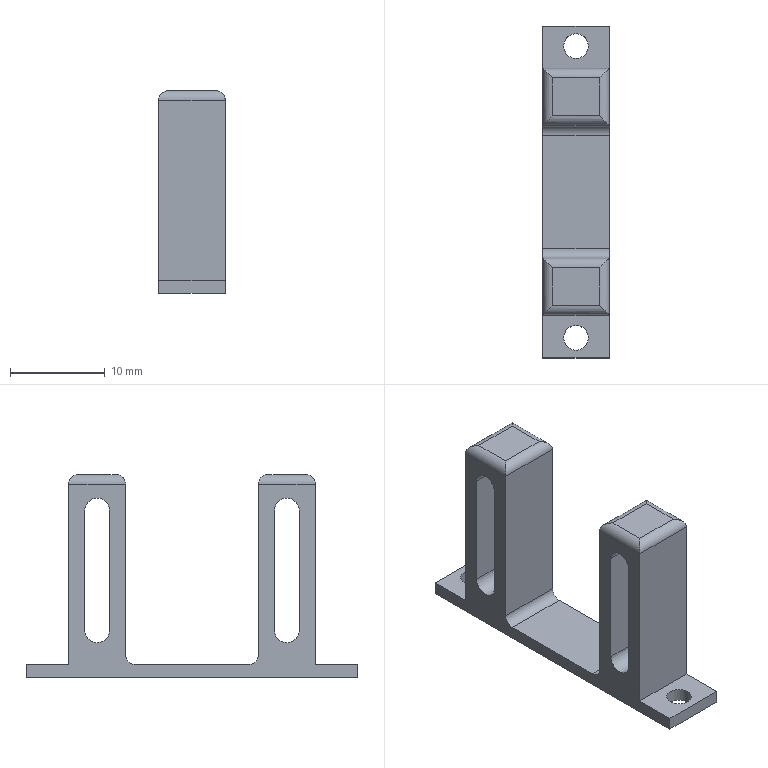Part | STEP file | Wytnij-wyci_gni_cie4 | 1 solid | 34 faces | box 7 x 35 x 21.379 mm | volume 1461 mm3 | plane 18 | cylinder 16 | commonest cylinder face diameters 2 x10 2.6 x6